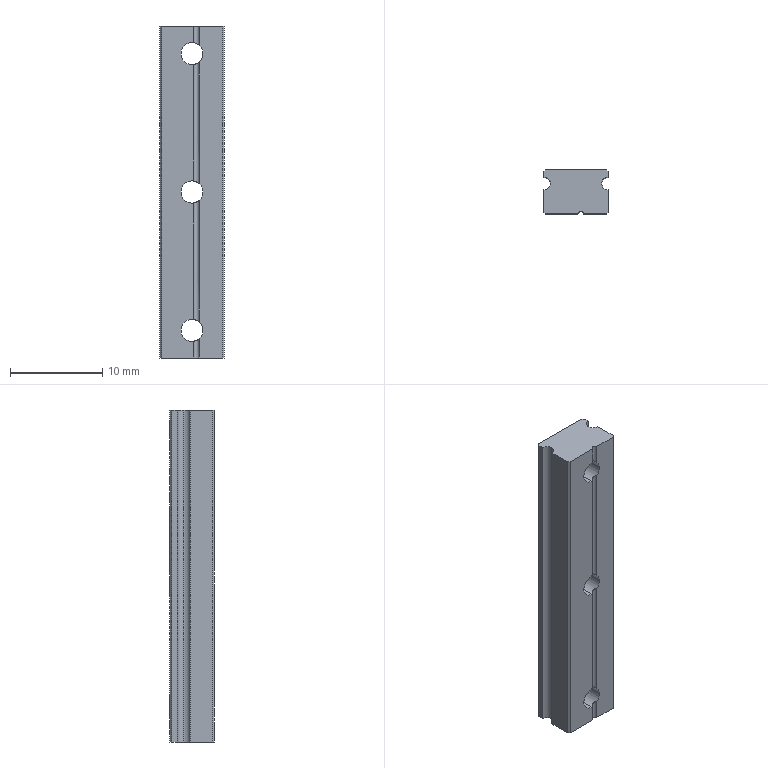Part | SolidWorks | features ICE 2, Extrusion 1, HoleWzd 1, LPattern 1 | 1 solid | 129 faces | box 7 x 4.8 x 36 mm | volume 1017 mm3 | plane 101 | cylinder 19 | spline 9 | commonest cylinder face diameters 2.4 x6 4.2 x6 0.6 x4 1.4 x3